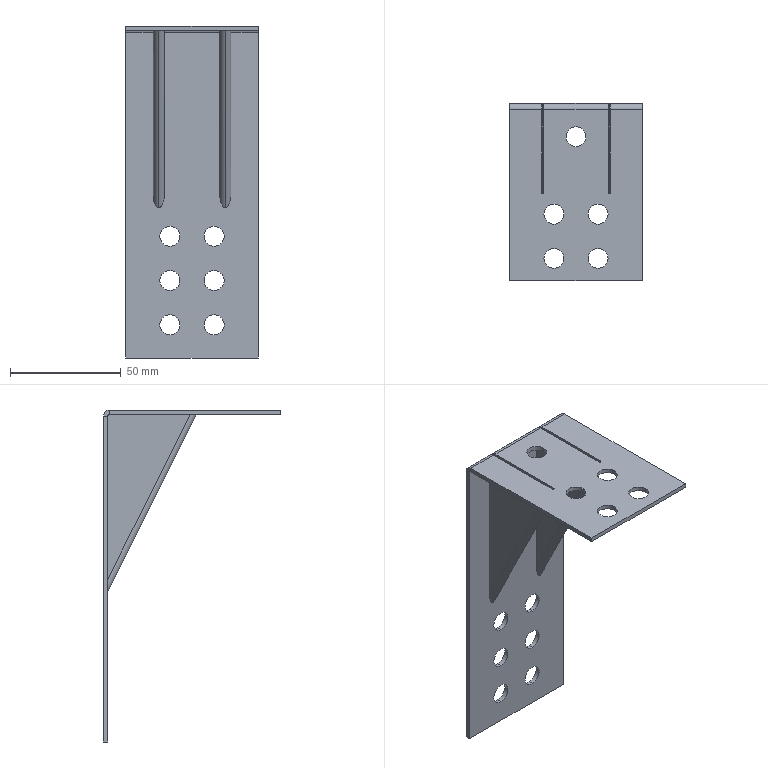Part | STEP file | MT-COMBO-119-S029 | 1 solid | 56 faces | box 60 x 80 x 150 mm | volume 38097 mm3 | cylinder 36 | plane 20 | commonest cylinder face diameters 9 x22 1 x4 5 x4 1.473 x3 5.473 x3